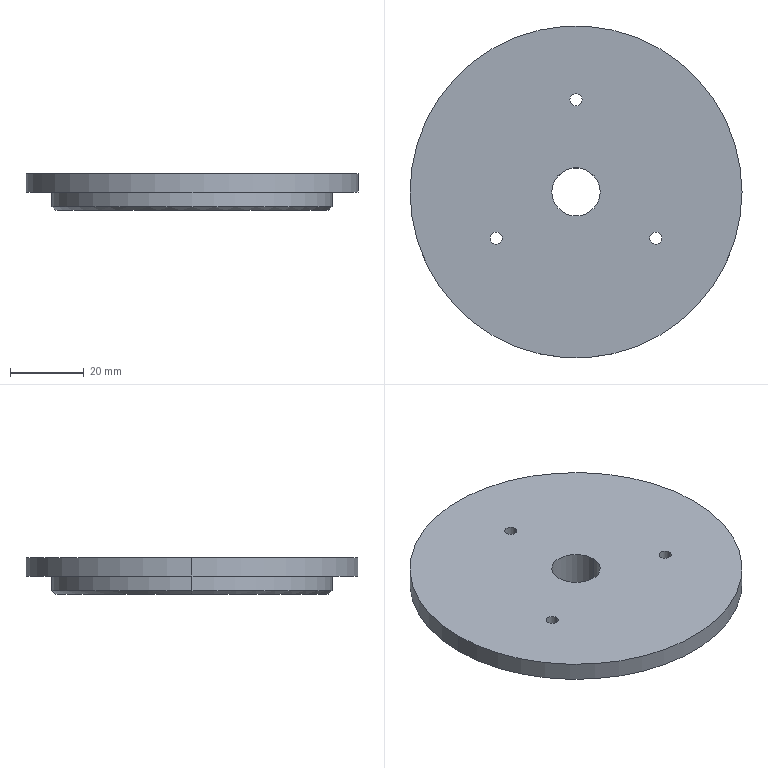Part | STEP file | 11-FG-B05511 | 1 solid | 17 faces | box 90 x 90 x 10 mm | volume 52768 mm3 | cylinder 12 | plane 3 | cone 2 | commonest cylinder face diameters 3.3 x6 13.1 x2 76 x2 90 x2
STEP:
#1=CARTESIAN_POINT('',(-23.301,-12.5,0.));
#2=VERTEX_POINT('',#1);
#3=CARTESIAN_POINT('',(-20.001,-12.5,0.));
#4=VERTEX_POINT('',#3);
#5=CARTESIAN_POINT('',(-21.651,-12.5,0.));
#6=DIRECTION('',(0.,0.,1.));
#7=DIRECTION('',(1.,0.,0.));
#8=AXIS2_PLACEMENT_3D('',#5,#6,#7);
#9=CIRCLE('',#8,1.65);
#10=EDGE_CURVE('',#2,#4,#9,.T.);
#11=ORIENTED_EDGE('',*,*,#10,.F.);
#12=CARTESIAN_POINT('',(-23.301,-12.5,10.));
#13=VERTEX_POINT('',#12);
#14=CARTESIAN_POINT('',(-23.301,-12.5,10.));
#15=DIRECTION('',(0.,0.,1.));
#16=VECTOR('',#15,1000.);
#17=LINE('',#14,#16);
#18=EDGE_CURVE('',#2,#13,#17,.T.);
#19=ORIENTED_EDGE('',*,*,#18,.T.);
#20=CARTESIAN_POINT('',(-20.001,-12.5,10.));
#21=VERTEX_POINT('',#20);
#22=CARTESIAN_POINT('',(-21.651,-12.5,10.));
#23=DIRECTION('',(0.,0.,1.));
#24=DIRECTION('',(1.,0.,0.));
#25=AXIS2_PLACEMENT_3D('',#22,#23,#24);
#26=CIRCLE('',#25,1.65);
#27=EDGE_CURVE('',#13,#21,#26,.T.);
#28=ORIENTED_EDGE('',*,*,#27,.T.);
#29=CARTESIAN_POINT('',(-20.001,-12.5,10.));
#30=DIRECTION('',(0.,0.,1.));
#31=VECTOR('',#30,1000.);
#32=LINE('',#29,#31);
#33=EDGE_CURVE('',#4,#21,#32,.T.);
#34=ORIENTED_EDGE('',*,*,#33,.F.);
#35=EDGE_LOOP('',(#11,#19,#28,#34));
#36=FACE_OUTER_BOUND('',#35,.T.);
#37=CARTESIAN_POINT('',(-21.651,-12.5,10.));
#38=DIRECTION('',(0.,0.,1.));
#39=DIRECTION('',(1.,0.,0.));
#40=AXIS2_PLACEMENT_3D('',#37,#38,#39);
#41=CYLINDRICAL_SURFACE('',#40,1.65);
#42=ADVANCED_FACE('',(#36),#41,.F.);
#43=CARTESIAN_POINT('',(20.001,-12.5,0.));
#44=VERTEX_POINT('',#43);
#45=CARTESIAN_POINT('',(23.301,-12.5,0.));
#46=VERTEX_POINT('',#45);
#47=CARTESIAN_POINT('',(21.651,-12.5,0.));
#48=DIRECTION('',(0.,0.,1.));
#49=DIRECTION('',(1.,0.,0.));
#50=AXIS2_PLACEMENT_3D('',#47,#48,#49);
#51=CIRCLE('',#50,1.65);
#52=EDGE_CURVE('',#44,#46,#51,.T.);
#53=ORIENTED_EDGE('',*,*,#52,.F.);
#54=CARTESIAN_POINT('',(20.001,-12.5,10.));
#55=VERTEX_POINT('',#54);
#56=CARTESIAN_POINT('',(20.001,-12.5,10.));
#57=DIRECTION('',(0.,0.,1.));
#58=VECTOR('',#57,1000.);
#59=LINE('',#56,#58);
#60=EDGE_CURVE('',#44,#55,#59,.T.);
#61=ORIENTED_EDGE('',*,*,#60,.T.);
#62=CARTESIAN_POINT('',(23.301,-12.5,10.));
#63=VERTEX_POINT('',#62);
#64=CARTESIAN_POINT('',(21.651,-12.5,10.));
#65=DIRECTION('',(0.,0.,1.));
#66=DIRECTION('',(1.,0.,0.));
#67=AXIS2_PLACEMENT_3D('',#64,#65,#66);
#68=CIRCLE('',#67,1.65);
#69=EDGE_CURVE('',#55,#63,#68,.T.);
#70=ORIENTED_EDGE('',*,*,#69,.T.);
#71=CARTESIAN_POINT('',(23.301,-12.5,10.));
#72=DIRECTION('',(0.,0.,1.));
#73=VECTOR('',#72,1000.);
#74=LINE('',#71,#73);
#75=EDGE_CURVE('',#46,#63,#74,.T.);
#76=ORIENTED_EDGE('',*,*,#75,.F.);
#77=EDGE_LOOP('',(#53,#61,#70,#76));
#78=FACE_OUTER_BOUND('',#77,.T.);
#79=CARTESIAN_POINT('',(21.651,-12.5,10.));
#80=DIRECTION('',(0.,0.,1.));
#81=DIRECTION('',(1.,0.,0.));
#82=AXIS2_PLACEMENT_3D('',#79,#80,#81);
#83=CYLINDRICAL_SURFACE('',#82,1.65);
#84=ADVANCED_FACE('',(#78),#83,.F.);
#85=CARTESIAN_POINT('',(-1.65,25.,0.));
#86=VERTEX_POINT('',#85);
#87=CARTESIAN_POINT('',(1.65,25.,0.));
#88=VERTEX_POINT('',#87);
#89=CARTESIAN_POINT('',(0.,25.,0.));
#90=DIRECTION('',(0.,0.,1.));
#91=DIRECTION('',(1.,0.,0.));
#92=AXIS2_PLACEMENT_3D('',#89,#90,#91);
#93=CIRCLE('',#92,1.65);
#94=EDGE_CURVE('',#86,#88,#93,.T.);
#95=ORIENTED_EDGE('',*,*,#94,.F.);
#96=CARTESIAN_POINT('',(-1.65,25.,10.));
#97=VERTEX_POINT('',#96);
#98=CARTESIAN_POINT('',(-1.65,25.,10.));
#99=DIRECTION('',(0.,0.,1.));
#100=VECTOR('',#99,1000.);
#101=LINE('',#98,#100);
#102=EDGE_CURVE('',#86,#97,#101,.T.);
#103=ORIENTED_EDGE('',*,*,#102,.T.);
#104=CARTESIAN_POINT('',(1.65,25.,10.));
#105=VERTEX_POINT('',#104);
#106=CARTESIAN_POINT('',(0.,25.,10.));
#107=DIRECTION('',(0.,0.,1.));
#108=DIRECTION('',(1.,0.,0.));
#109=AXIS2_PLACEMENT_3D('',#106,#107,#108);
#110=CIRCLE('',#109,1.65);
#111=EDGE_CURVE('',#97,#105,#110,.T.);
#112=ORIENTED_EDGE('',*,*,#111,.T.);
#113=CARTESIAN_POINT('',(1.65,25.,10.));
#114=DIRECTION('',(0.,0.,1.));
#115=VECTOR('',#114,1000.);
#116=LINE('',#113,#115);
#117=EDGE_CURVE('',#88,#105,#116,.T.);
#118=ORIENTED_EDGE('',*,*,#117,.F.);
#119=EDGE_LOOP('',(#95,#103,#112,#118));
#120=FACE_OUTER_BOUND('',#119,.T.);
#121=CARTESIAN_POINT('',(0.,25.,10.));
#122=DIRECTION('',(0.,0.,1.));
#123=DIRECTION('',(1.,0.,0.));
#124=AXIS2_PLACEMENT_3D('',#121,#122,#123);
#125=CYLINDRICAL_SURFACE('',#124,1.65);
#126=ADVANCED_FACE('',(#120),#125,.F.);
#127=CARTESIAN_POINT('',(6.55,0.,10.));
#128=VERTEX_POINT('',#127);
#129=CARTESIAN_POINT('',(-6.55,0.,10.));
#130=VERTEX_POINT('',#129);
#131=CARTESIAN_POINT('',(0.,0.,10.));
#132=DIRECTION('',(0.,0.,-1.));
#133=DIRECTION('',(-1.,0.,0.));
#134=AXIS2_PLACEMENT_3D('',#131,#132,#133);
#135=CIRCLE('',#134,6.55);
#136=EDGE_CURVE('',#128,#130,#135,.T.);
#137=ORIENTED_EDGE('',*,*,#136,.F.);
#138=CARTESIAN_POINT('',(6.55,0.,0.));
#139=VERTEX_POINT('',#138);
#140=CARTESIAN_POINT('',(6.55,0.,10.));
#141=DIRECTION('',(0.,0.,-1.));
#142=VECTOR('',#141,1000.);
#143=LINE('',#140,#142);
#144=EDGE_CURVE('',#128,#139,#143,.T.);
#145=ORIENTED_EDGE('',*,*,#144,.T.);
#146=CARTESIAN_POINT('',(-6.55,0.,0.));
#147=VERTEX_POINT('',#146);
#148=CARTESIAN_POINT('',(0.,0.,0.));
#149=DIRECTION('',(0.,0.,-1.));
#150=DIRECTION('',(-1.,0.,0.));
#151=AXIS2_PLACEMENT_3D('',#148,#149,#150);
#152=CIRCLE('',#151,6.55);
#153=EDGE_CURVE('',#139,#147,#152,.T.);
#154=ORIENTED_EDGE('',*,*,#153,.T.);
#155=CARTESIAN_POINT('',(-6.55,0.,10.));
#156=DIRECTION('',(0.,0.,-1.));
#157=VECTOR('',#156,1000.);
#158=LINE('',#155,#157);
#159=EDGE_CURVE('',#130,#147,#158,.T.);
#160=ORIENTED_EDGE('',*,*,#159,.F.);
#161=EDGE_LOOP('',(#137,#145,#154,#160));
#162=FACE_OUTER_BOUND('',#161,.T.);
#163=CARTESIAN_POINT('',(0.,0.,10.));
#164=DIRECTION('',(0.,0.,-1.));
#165=DIRECTION('',(-1.,0.,0.));
#166=AXIS2_PLACEMENT_3D('',#163,#164,#165);
#167=CYLINDRICAL_SURFACE('',#166,6.55);
#168=ADVANCED_FACE('',(#162),#167,.F.);
#169=CARTESIAN_POINT('',(-37.,0.,0.));
#170=VERTEX_POINT('',#169);
#171=CARTESIAN_POINT('',(37.,0.,0.));
#172=VERTEX_POINT('',#171);
#173=CARTESIAN_POINT('',(0.,0.,0.));
#174=DIRECTION('',(0.,0.,-1.));
#175=DIRECTION('',(1.,0.,0.));
#176=AXIS2_PLACEMENT_3D('',#173,#174,#175);
#177=CIRCLE('',#176,37.);
#178=EDGE_CURVE('',#170,#172,#177,.T.);
#179=ORIENTED_EDGE('',*,*,#178,.F.);
#180=CARTESIAN_POINT('',(-38.,0.,1.));
#181=VERTEX_POINT('',#180);
#182=CARTESIAN_POINT('',(-38.,0.,1.));
#183=DIRECTION('',(-0.7071,0.,0.7071));
#184=VECTOR('',#183,1000.);
#185=LINE('',#182,#184);
#186=EDGE_CURVE('',#170,#181,#185,.T.);
#187=ORIENTED_EDGE('',*,*,#186,.T.);
#188=CARTESIAN_POINT('',(38.,0.,1.));
#189=VERTEX_POINT('',#188);
#190=CARTESIAN_POINT('',(0.,0.,1.));
#191=DIRECTION('',(0.,0.,1.));
#192=DIRECTION('',(1.,0.,0.));
#193=AXIS2_PLACEMENT_3D('',#190,#191,#192);
#194=CIRCLE('',#193,38.);
#195=EDGE_CURVE('',#189,#181,#194,.T.);
#196=ORIENTED_EDGE('',*,*,#195,.F.);
#197=CARTESIAN_POINT('',(38.,0.,1.));
#198=DIRECTION('',(0.7071,0.,0.7071));
#199=VECTOR('',#198,1000.);
#200=LINE('',#197,#199);
#201=EDGE_CURVE('',#172,#189,#200,.T.);
#202=ORIENTED_EDGE('',*,*,#201,.F.);
#203=EDGE_LOOP('',(#179,#187,#196,#202));
#204=FACE_OUTER_BOUND('',#203,.T.);
#205=CARTESIAN_POINT('',(0.,0.,1.));
#206=DIRECTION('',(0.,0.,1.));
#207=DIRECTION('',(1.,0.,0.));
#208=AXIS2_PLACEMENT_3D('',#205,#206,#207);
#209=CONICAL_SURFACE('',#208,38.,0.7854);
#210=ADVANCED_FACE('',(#204),#209,.T.);
#211=CARTESIAN_POINT('',(45.,0.,10.));
#212=VERTEX_POINT('',#211);
#213=CARTESIAN_POINT('',(-45.,0.,10.));
#214=VERTEX_POINT('',#213);
#215=CARTESIAN_POINT('',(0.,0.,10.));
#216=DIRECTION('',(0.,0.,1.));
#217=DIRECTION('',(1.,0.,0.));
#218=AXIS2_PLACEMENT_3D('',#215,#216,#217);
#219=CIRCLE('',#218,45.);
#220=EDGE_CURVE('',#212,#214,#219,.T.);
#221=ORIENTED_EDGE('',*,*,#220,.F.);
#222=CARTESIAN_POINT('',(45.,0.,5.));
#223=VERTEX_POINT('',#222);
#224=CARTESIAN_POINT('',(45.,0.,10.));
#225=DIRECTION('',(0.,0.,-1.));
#226=VECTOR('',#225,1000.);
#227=LINE('',#224,#226);
#228=EDGE_CURVE('',#212,#223,#227,.T.);
#229=ORIENTED_EDGE('',*,*,#228,.T.);
#230=CARTESIAN_POINT('',(-45.,0.,5.));
#231=VERTEX_POINT('',#230);
#232=CARTESIAN_POINT('',(0.,0.,5.));
#233=DIRECTION('',(0.,0.,1.));
#234=DIRECTION('',(1.,0.,0.));
#235=AXIS2_PLACEMENT_3D('',#232,#233,#234);
#236=CIRCLE('',#235,45.);
#237=EDGE_CURVE('',#223,#231,#236,.T.);
#238=ORIENTED_EDGE('',*,*,#237,.T.);
#239=CARTESIAN_POINT('',(-45.,0.,10.));
#240=DIRECTION('',(0.,0.,-1.));
#241=VECTOR('',#240,1000.);
#242=LINE('',#239,#241);
#243=EDGE_CURVE('',#214,#231,#242,.T.);
#244=ORIENTED_EDGE('',*,*,#243,.F.);
#245=EDGE_LOOP('',(#221,#229,#238,#244));
#246=FACE_OUTER_BOUND('',#245,.T.);
#247=CARTESIAN_POINT('',(0.,0.,10.));
#248=DIRECTION('',(0.,0.,-1.));
#249=DIRECTION('',(-1.,0.,0.));
#250=AXIS2_PLACEMENT_3D('',#247,#248,#249);
#251=CYLINDRICAL_SURFACE('',#250,45.);
#252=ADVANCED_FACE('',(#246),#251,.T.);
#253=CARTESIAN_POINT('',(38.,0.,5.));
#254=VERTEX_POINT('',#253);
#255=CARTESIAN_POINT('',(-38.,0.,5.));
#256=VERTEX_POINT('',#255);
#257=CARTESIAN_POINT('',(0.,0.,5.));
#258=DIRECTION('',(0.,0.,1.));
#259=DIRECTION('',(1.,0.,0.));
#260=AXIS2_PLACEMENT_3D('',#257,#258,#259);
#261=CIRCLE('',#260,38.);
#262=EDGE_CURVE('',#254,#256,#261,.T.);
#263=ORIENTED_EDGE('',*,*,#262,.F.);
#264=CARTESIAN_POINT('',(38.,0.,5.));
#265=DIRECTION('',(0.,0.,-1.));
#266=VECTOR('',#265,1000.);
#267=LINE('',#264,#266);
#268=EDGE_CURVE('',#254,#189,#267,.T.);
#269=ORIENTED_EDGE('',*,*,#268,.T.);
#270=ORIENTED_EDGE('',*,*,#195,.T.);
#271=CARTESIAN_POINT('',(-38.,0.,5.));
#272=DIRECTION('',(0.,0.,-1.));
#273=VECTOR('',#272,1000.);
#274=LINE('',#271,#273);
#275=EDGE_CURVE('',#256,#181,#274,.T.);
#276=ORIENTED_EDGE('',*,*,#275,.F.);
#277=EDGE_LOOP('',(#263,#269,#270,#276));
#278=FACE_OUTER_BOUND('',#277,.T.);
#279=CARTESIAN_POINT('',(0.,0.,5.));
#280=DIRECTION('',(0.,0.,-1.));
#281=DIRECTION('',(-1.,0.,0.));
#282=AXIS2_PLACEMENT_3D('',#279,#280,#281);
#283=CYLINDRICAL_SURFACE('',#282,38.);
#284=ADVANCED_FACE('',(#278),#283,.T.);
#285=ORIENTED_EDGE('',*,*,#268,.F.);
#286=CARTESIAN_POINT('',(0.,0.,5.));
#287=DIRECTION('',(0.,0.,1.));
#288=DIRECTION('',(1.,0.,0.));
#289=AXIS2_PLACEMENT_3D('',#286,#287,#288);
#290=CIRCLE('',#289,38.);
#291=EDGE_CURVE('',#256,#254,#290,.T.);
#292=ORIENTED_EDGE('',*,*,#291,.F.);
#293=ORIENTED_EDGE('',*,*,#275,.T.);
#294=CARTESIAN_POINT('',(0.,0.,1.));
#295=DIRECTION('',(0.,0.,1.));
#296=DIRECTION('',(1.,0.,0.));
#297=AXIS2_PLACEMENT_3D('',#294,#295,#296);
#298=CIRCLE('',#297,38.);
#299=EDGE_CURVE('',#181,#189,#298,.T.);
#300=ORIENTED_EDGE('',*,*,#299,.T.);
#301=EDGE_LOOP('',(#285,#292,#293,#300));
#302=FACE_OUTER_BOUND('',#301,.T.);
#303=CARTESIAN_POINT('',(0.,0.,5.));
#304=DIRECTION('',(0.,0.,-1.));
#305=DIRECTION('',(-1.,0.,0.));
#306=AXIS2_PLACEMENT_3D('',#303,#304,#305);
#307=CYLINDRICAL_SURFACE('',#306,38.);
#308=ADVANCED_FACE('',(#302),#307,.T.);
#309=CARTESIAN_POINT('',(-21.651,-12.5,0.));
#310=DIRECTION('',(0.,0.,1.));
#311=DIRECTION('',(1.,0.,0.));
#312=AXIS2_PLACEMENT_3D('',#309,#310,#311);
#313=CIRCLE('',#312,1.65);
#314=EDGE_CURVE('',#4,#2,#313,.T.);
#315=ORIENTED_EDGE('',*,*,#314,.T.);
#316=ORIENTED_EDGE('',*,*,#10,.T.);
#317=EDGE_LOOP('',(#315,#316));
#318=FACE_BOUND('',#317,.T.);
#319=CARTESIAN_POINT('',(21.651,-12.5,0.));
#320=DIRECTION('',(0.,0.,1.));
#321=DIRECTION('',(1.,0.,0.));
#322=AXIS2_PLACEMENT_3D('',#319,#320,#321);
#323=CIRCLE('',#322,1.65);
#324=EDGE_CURVE('',#46,#44,#323,.T.);
#325=ORIENTED_EDGE('',*,*,#324,.T.);
#326=ORIENTED_EDGE('',*,*,#52,.T.);
#327=EDGE_LOOP('',(#325,#326));
#328=FACE_BOUND('',#327,.T.);
#329=CARTESIAN_POINT('',(0.,25.,0.));
#330=DIRECTION('',(0.,0.,1.));
#331=DIRECTION('',(1.,0.,0.));
#332=AXIS2_PLACEMENT_3D('',#329,#330,#331);
#333=CIRCLE('',#332,1.65);
#334=EDGE_CURVE('',#88,#86,#333,.T.);
#335=ORIENTED_EDGE('',*,*,#334,.T.);
#336=ORIENTED_EDGE('',*,*,#94,.T.);
#337=EDGE_LOOP('',(#335,#336));
#338=FACE_BOUND('',#337,.T.);
#339=CARTESIAN_POINT('',(0.,0.,0.));
#340=DIRECTION('',(0.,0.,-1.));
#341=DIRECTION('',(-1.,0.,0.));
#342=AXIS2_PLACEMENT_3D('',#339,#340,#341);
#343=CIRCLE('',#342,6.55);
#344=EDGE_CURVE('',#147,#139,#343,.T.);
#345=ORIENTED_EDGE('',*,*,#344,.F.);
#346=ORIENTED_EDGE('',*,*,#153,.F.);
#347=EDGE_LOOP('',(#345,#346));
#348=FACE_BOUND('',#347,.T.);
#349=CARTESIAN_POINT('',(0.,0.,0.));
#350=DIRECTION('',(0.,0.,-1.));
#351=DIRECTION('',(1.,0.,0.));
#352=AXIS2_PLACEMENT_3D('',#349,#350,#351);
#353=CIRCLE('',#352,37.);
#354=EDGE_CURVE('',#172,#170,#353,.T.);
#355=ORIENTED_EDGE('',*,*,#354,.T.);
#356=ORIENTED_EDGE('',*,*,#178,.T.);
#357=EDGE_LOOP('',(#355,#356));
#358=FACE_OUTER_BOUND('',#357,.T.);
#359=CARTESIAN_POINT('',(0.,0.,0.));
#360=DIRECTION('',(0.,0.,1.));
#361=DIRECTION('',(1.,0.,0.));
#362=AXIS2_PLACEMENT_3D('',#359,#360,#361);
#363=PLANE('',#362);
#364=ADVANCED_FACE('',(#318,#328,#338,#348,#358),#363,.F.);
#365=CARTESIAN_POINT('',(0.,0.,5.));
#366=DIRECTION('',(0.,0.,1.));
#367=DIRECTION('',(1.,0.,0.));
#368=AXIS2_PLACEMENT_3D('',#365,#366,#367);
#369=CIRCLE('',#368,45.);
#370=EDGE_CURVE('',#231,#223,#369,.T.);
#371=ORIENTED_EDGE('',*,*,#370,.F.);
#372=ORIENTED_EDGE('',*,*,#237,.F.);
#373=EDGE_LOOP('',(#371,#372));
#374=FACE_OUTER_BOUND('',#373,.T.);
#375=ORIENTED_EDGE('',*,*,#291,.T.);
#376=ORIENTED_EDGE('',*,*,#262,.T.);
#377=EDGE_LOOP('',(#375,#376));
#378=FACE_BOUND('',#377,.T.);
#379=CARTESIAN_POINT('',(0.,0.,5.));
#380=DIRECTION('',(0.,0.,1.));
#381=DIRECTION('',(1.,0.,0.));
#382=AXIS2_PLACEMENT_3D('',#379,#380,#381);
#383=PLANE('',#382);
#384=ADVANCED_FACE('',(#374,#378),#383,.F.);
#385=ORIENTED_EDGE('',*,*,#228,.F.);
#386=CARTESIAN_POINT('',(0.,0.,10.));
#387=DIRECTION('',(0.,0.,1.));
#388=DIRECTION('',(1.,0.,0.));
#389=AXIS2_PLACEMENT_3D('',#386,#387,#388);
#390=CIRCLE('',#389,45.);
#391=EDGE_CURVE('',#214,#212,#390,.T.);
#392=ORIENTED_EDGE('',*,*,#391,.F.);
#393=ORIENTED_EDGE('',*,*,#243,.T.);
#394=ORIENTED_EDGE('',*,*,#370,.T.);
#395=EDGE_LOOP('',(#385,#392,#393,#394));
#396=FACE_OUTER_BOUND('',#395,.T.);
#397=CARTESIAN_POINT('',(0.,0.,10.));
#398=DIRECTION('',(0.,0.,-1.));
#399=DIRECTION('',(-1.,0.,0.));
#400=AXIS2_PLACEMENT_3D('',#397,#398,#399);
#401=CYLINDRICAL_SURFACE('',#400,45.);
#402=ADVANCED_FACE('',(#396),#401,.T.);
#403=CARTESIAN_POINT('',(-21.651,-12.5,10.));
#404=DIRECTION('',(0.,0.,1.));
#405=DIRECTION('',(1.,0.,0.));
#406=AXIS2_PLACEMENT_3D('',#403,#404,#405);
#407=CIRCLE('',#406,1.65);
#408=EDGE_CURVE('',#21,#13,#407,.T.);
#409=ORIENTED_EDGE('',*,*,#408,.F.);
#410=ORIENTED_EDGE('',*,*,#27,.F.);
#411=EDGE_LOOP('',(#409,#410));
#412=FACE_BOUND('',#411,.T.);
#413=CARTESIAN_POINT('',(21.651,-12.5,10.));
#414=DIRECTION('',(0.,0.,1.));
#415=DIRECTION('',(1.,0.,0.));
#416=AXIS2_PLACEMENT_3D('',#413,#414,#415);
#417=CIRCLE('',#416,1.65);
#418=EDGE_CURVE('',#63,#55,#417,.T.);
#419=ORIENTED_EDGE('',*,*,#418,.F.);
#420=ORIENTED_EDGE('',*,*,#69,.F.);
#421=EDGE_LOOP('',(#419,#420));
#422=FACE_BOUND('',#421,.T.);
#423=CARTESIAN_POINT('',(0.,25.,10.));
#424=DIRECTION('',(0.,0.,1.));
#425=DIRECTION('',(1.,0.,0.));
#426=AXIS2_PLACEMENT_3D('',#423,#424,#425);
#427=CIRCLE('',#426,1.65);
#428=EDGE_CURVE('',#105,#97,#427,.T.);
#429=ORIENTED_EDGE('',*,*,#428,.F.);
#430=ORIENTED_EDGE('',*,*,#111,.F.);
#431=EDGE_LOOP('',(#429,#430));
#432=FACE_BOUND('',#431,.T.);
#433=CARTESIAN_POINT('',(0.,0.,10.));
#434=DIRECTION('',(0.,0.,-1.));
#435=DIRECTION('',(-1.,0.,0.));
#436=AXIS2_PLACEMENT_3D('',#433,#434,#435);
#437=CIRCLE('',#436,6.55);
#438=EDGE_CURVE('',#130,#128,#437,.T.);
#439=ORIENTED_EDGE('',*,*,#438,.T.);
#440=ORIENTED_EDGE('',*,*,#136,.T.);
#441=EDGE_LOOP('',(#439,#440));
#442=FACE_BOUND('',#441,.T.);
#443=ORIENTED_EDGE('',*,*,#391,.T.);
#444=ORIENTED_EDGE('',*,*,#220,.T.);
#445=EDGE_LOOP('',(#443,#444));
#446=FACE_OUTER_BOUND('',#445,.T.);
#447=CARTESIAN_POINT('',(0.,0.,10.));
#448=DIRECTION('',(0.,0.,1.));
#449=DIRECTION('',(1.,0.,0.));
#450=AXIS2_PLACEMENT_3D('',#447,#448,#449);
#451=PLANE('',#450);
#452=ADVANCED_FACE('',(#412,#422,#432,#442,#446),#451,.T.);
#453=ORIENTED_EDGE('',*,*,#186,.F.);
#454=ORIENTED_EDGE('',*,*,#354,.F.);
#455=ORIENTED_EDGE('',*,*,#201,.T.);
#456=ORIENTED_EDGE('',*,*,#299,.F.);
#457=EDGE_LOOP('',(#453,#454,#455,#456));
#458=FACE_OUTER_BOUND('',#457,.T.);
#459=CARTESIAN_POINT('',(0.,0.,1.));
#460=DIRECTION('',(0.,0.,1.));
#461=DIRECTION('',(1.,0.,0.));
#462=AXIS2_PLACEMENT_3D('',#459,#460,#461);
#463=CONICAL_SURFACE('',#462,38.,0.7854);
#464=ADVANCED_FACE('',(#458),#463,.T.);
#465=ORIENTED_EDGE('',*,*,#144,.F.);
#466=ORIENTED_EDGE('',*,*,#438,.F.);
#467=ORIENTED_EDGE('',*,*,#159,.T.);
#468=ORIENTED_EDGE('',*,*,#344,.T.);
#469=EDGE_LOOP('',(#465,#466,#467,#468));
#470=FACE_OUTER_BOUND('',#469,.T.);
#471=CARTESIAN_POINT('',(0.,0.,10.));
#472=DIRECTION('',(0.,0.,-1.));
#473=DIRECTION('',(-1.,0.,0.));
#474=AXIS2_PLACEMENT_3D('',#471,#472,#473);
#475=CYLINDRICAL_SURFACE('',#474,6.55);
#476=ADVANCED_FACE('',(#470),#475,.F.);
#477=ORIENTED_EDGE('',*,*,#102,.F.);
#478=ORIENTED_EDGE('',*,*,#334,.F.);
#479=ORIENTED_EDGE('',*,*,#117,.T.);
#480=ORIENTED_EDGE('',*,*,#428,.T.);
#481=EDGE_LOOP('',(#477,#478,#479,#480));
#482=FACE_OUTER_BOUND('',#481,.T.);
#483=CARTESIAN_POINT('',(0.,25.,10.));
#484=DIRECTION('',(0.,0.,1.));
#485=DIRECTION('',(1.,0.,0.));
#486=AXIS2_PLACEMENT_3D('',#483,#484,#485);
#487=CYLINDRICAL_SURFACE('',#486,1.65);
#488=ADVANCED_FACE('',(#482),#487,.F.);
#489=ORIENTED_EDGE('',*,*,#60,.F.);
#490=ORIENTED_EDGE('',*,*,#324,.F.);
#491=ORIENTED_EDGE('',*,*,#75,.T.);
#492=ORIENTED_EDGE('',*,*,#418,.T.);
#493=EDGE_LOOP('',(#489,#490,#491,#492));
#494=FACE_OUTER_BOUND('',#493,.T.);
#495=CARTESIAN_POINT('',(21.651,-12.5,10.));
#496=DIRECTION('',(0.,0.,1.));
#497=DIRECTION('',(1.,0.,0.));
#498=AXIS2_PLACEMENT_3D('',#495,#496,#497);
#499=CYLINDRICAL_SURFACE('',#498,1.65);
#500=ADVANCED_FACE('',(#494),#499,.F.);
#501=ORIENTED_EDGE('',*,*,#18,.F.);
#502=ORIENTED_EDGE('',*,*,#314,.F.);
#503=ORIENTED_EDGE('',*,*,#33,.T.);
#504=ORIENTED_EDGE('',*,*,#408,.T.);
#505=EDGE_LOOP('',(#501,#502,#503,#504));
#506=FACE_OUTER_BOUND('',#505,.T.);
#507=CARTESIAN_POINT('',(-21.651,-12.5,10.));
#508=DIRECTION('',(0.,0.,1.));
#509=DIRECTION('',(1.,0.,0.));
#510=AXIS2_PLACEMENT_3D('',#507,#508,#509);
#511=CYLINDRICAL_SURFACE('',#510,1.65);
#512=ADVANCED_FACE('',(#506),#511,.F.);
#513=CLOSED_SHELL('',(#42,#84,#126,#168,#210,#252,#284,#308,#364,#384,#402,#452,#464,#476,#488,#500,#512));
#514=MANIFOLD_SOLID_BREP('',#513);
#515=CARTESIAN_POINT('',(0.,0.,0.));
#516=DIRECTION('',(0.,0.,1.));
#517=DIRECTION('',(1.,0.,0.));
#518=AXIS2_PLACEMENT_3D('',#515,#516,#517);
#519=(LENGTH_UNIT()NAMED_UNIT(*)SI_UNIT(.MILLI.,.METRE.));
#520=UNCERTAINTY_MEASURE_WITH_UNIT(LENGTH_MEASURE(0.00001),#519,'','');
#521=(NAMED_UNIT(*)PLANE_ANGLE_UNIT()SI_UNIT($,.RADIAN.));
#522=(NAMED_UNIT(*)SI_UNIT($,.STERADIAN.)SOLID_ANGLE_UNIT());
#523=(GEOMETRIC_REPRESENTATION_CONTEXT(3)GLOBAL_UNCERTAINTY_ASSIGNED_CONTEXT((#520))GLOBAL_UNIT_ASSIGNED_CONTEXT((#519,#521,#522))REPRESENTATION_CONTEXT('',''));
#524=ADVANCED_BREP_SHAPE_REPRESENTATION('',(#514,#518),#523);